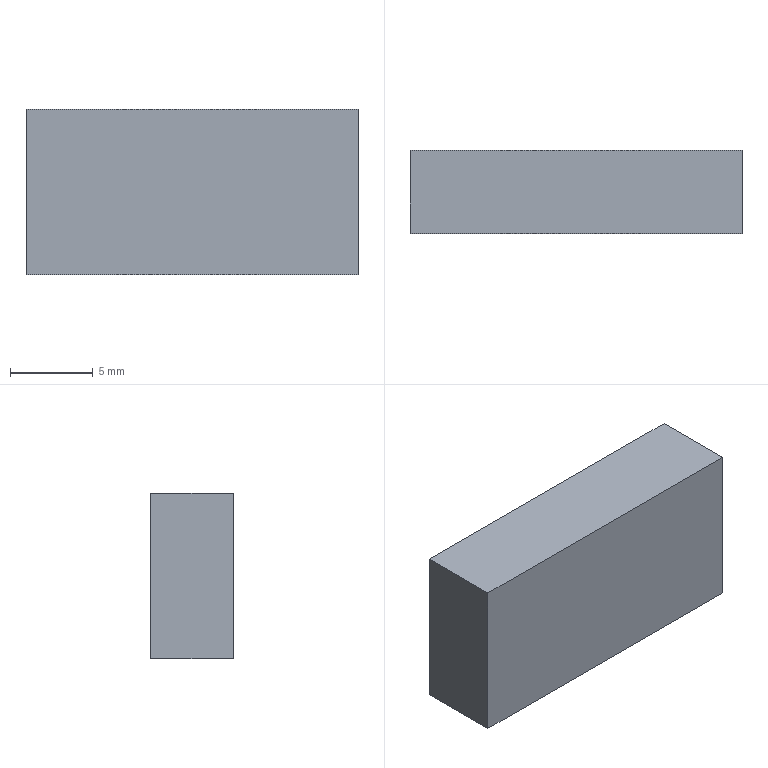Part | SolidWorks | features Extrusion 1 | 1 solid | 6 faces | box 20 x 5 x 10 mm | volume 1000 mm3 | plane 6
STEP:
#1=CARTESIAN_POINT('',(10.,0.,5.));
#2=VERTEX_POINT('',#1);
#3=CARTESIAN_POINT('',(10.,0.,-5.));
#4=VERTEX_POINT('',#3);
#5=CARTESIAN_POINT('',(10.,0.,5.));
#6=DIRECTION('',(0.,0.,-1.));
#7=VECTOR('',#6,1000.);
#8=LINE('',#5,#7);
#9=EDGE_CURVE('',#2,#4,#8,.T.);
#10=ORIENTED_EDGE('',*,*,#9,.T.);
#11=CARTESIAN_POINT('',(10.,5.,-5.));
#12=VERTEX_POINT('',#11);
#13=CARTESIAN_POINT('',(10.,5.,-5.));
#14=DIRECTION('',(0.,-1.,0.));
#15=VECTOR('',#14,1000.);
#16=LINE('',#13,#15);
#17=EDGE_CURVE('',#12,#4,#16,.T.);
#18=ORIENTED_EDGE('',*,*,#17,.F.);
#19=CARTESIAN_POINT('',(10.,5.,5.));
#20=VERTEX_POINT('',#19);
#21=CARTESIAN_POINT('',(10.,5.,5.));
#22=DIRECTION('',(0.,0.,-1.));
#23=VECTOR('',#22,1000.);
#24=LINE('',#21,#23);
#25=EDGE_CURVE('',#20,#12,#24,.T.);
#26=ORIENTED_EDGE('',*,*,#25,.F.);
#27=CARTESIAN_POINT('',(10.,5.,5.));
#28=DIRECTION('',(0.,-1.,0.));
#29=VECTOR('',#28,1000.);
#30=LINE('',#27,#29);
#31=EDGE_CURVE('',#20,#2,#30,.T.);
#32=ORIENTED_EDGE('',*,*,#31,.T.);
#33=EDGE_LOOP('',(#10,#18,#26,#32));
#34=FACE_OUTER_BOUND('',#33,.T.);
#35=CARTESIAN_POINT('',(10.,5.,5.));
#36=DIRECTION('',(-1.,0.,0.));
#37=DIRECTION('',(0.,0.,1.));
#38=AXIS2_PLACEMENT_3D('',#35,#36,#37);
#39=PLANE('',#38);
#40=ADVANCED_FACE('',(#34),#39,.F.);
#41=CARTESIAN_POINT('',(-10.,0.,-5.));
#42=VERTEX_POINT('',#41);
#43=CARTESIAN_POINT('',(-10.,0.,-5.));
#44=DIRECTION('',(-1.,0.,0.));
#45=VECTOR('',#44,1000.);
#46=LINE('',#43,#45);
#47=EDGE_CURVE('',#4,#42,#46,.T.);
#48=ORIENTED_EDGE('',*,*,#47,.T.);
#49=CARTESIAN_POINT('',(-10.,5.,-5.));
#50=VERTEX_POINT('',#49);
#51=CARTESIAN_POINT('',(-10.,5.,-5.));
#52=DIRECTION('',(0.,-1.,0.));
#53=VECTOR('',#52,1000.);
#54=LINE('',#51,#53);
#55=EDGE_CURVE('',#50,#42,#54,.T.);
#56=ORIENTED_EDGE('',*,*,#55,.F.);
#57=CARTESIAN_POINT('',(-10.,5.,-5.));
#58=DIRECTION('',(-1.,0.,0.));
#59=VECTOR('',#58,1000.);
#60=LINE('',#57,#59);
#61=EDGE_CURVE('',#12,#50,#60,.T.);
#62=ORIENTED_EDGE('',*,*,#61,.F.);
#63=ORIENTED_EDGE('',*,*,#17,.T.);
#64=EDGE_LOOP('',(#48,#56,#62,#63));
#65=FACE_OUTER_BOUND('',#64,.T.);
#66=CARTESIAN_POINT('',(-10.,5.,-5.));
#67=DIRECTION('',(0.,0.,1.));
#68=DIRECTION('',(1.,0.,0.));
#69=AXIS2_PLACEMENT_3D('',#66,#67,#68);
#70=PLANE('',#69);
#71=ADVANCED_FACE('',(#65),#70,.F.);
#72=CARTESIAN_POINT('',(-10.,0.,5.));
#73=VERTEX_POINT('',#72);
#74=CARTESIAN_POINT('',(-10.,0.,5.));
#75=DIRECTION('',(0.,0.,1.));
#76=VECTOR('',#75,1000.);
#77=LINE('',#74,#76);
#78=EDGE_CURVE('',#42,#73,#77,.T.);
#79=ORIENTED_EDGE('',*,*,#78,.T.);
#80=CARTESIAN_POINT('',(-10.,5.,5.));
#81=VERTEX_POINT('',#80);
#82=CARTESIAN_POINT('',(-10.,5.,5.));
#83=DIRECTION('',(0.,-1.,0.));
#84=VECTOR('',#83,1000.);
#85=LINE('',#82,#84);
#86=EDGE_CURVE('',#81,#73,#85,.T.);
#87=ORIENTED_EDGE('',*,*,#86,.F.);
#88=CARTESIAN_POINT('',(-10.,5.,5.));
#89=DIRECTION('',(0.,0.,1.));
#90=VECTOR('',#89,1000.);
#91=LINE('',#88,#90);
#92=EDGE_CURVE('',#50,#81,#91,.T.);
#93=ORIENTED_EDGE('',*,*,#92,.F.);
#94=ORIENTED_EDGE('',*,*,#55,.T.);
#95=EDGE_LOOP('',(#79,#87,#93,#94));
#96=FACE_OUTER_BOUND('',#95,.T.);
#97=CARTESIAN_POINT('',(-10.,5.,5.));
#98=DIRECTION('',(1.,0.,0.));
#99=DIRECTION('',(0.,0.,-1.));
#100=AXIS2_PLACEMENT_3D('',#97,#98,#99);
#101=PLANE('',#100);
#102=ADVANCED_FACE('',(#96),#101,.F.);
#103=CARTESIAN_POINT('',(-10.,0.,5.));
#104=DIRECTION('',(1.,0.,0.));
#105=VECTOR('',#104,1000.);
#106=LINE('',#103,#105);
#107=EDGE_CURVE('',#73,#2,#106,.T.);
#108=ORIENTED_EDGE('',*,*,#107,.T.);
#109=ORIENTED_EDGE('',*,*,#31,.F.);
#110=CARTESIAN_POINT('',(-10.,5.,5.));
#111=DIRECTION('',(1.,0.,0.));
#112=VECTOR('',#111,1000.);
#113=LINE('',#110,#112);
#114=EDGE_CURVE('',#81,#20,#113,.T.);
#115=ORIENTED_EDGE('',*,*,#114,.F.);
#116=ORIENTED_EDGE('',*,*,#86,.T.);
#117=EDGE_LOOP('',(#108,#109,#115,#116));
#118=FACE_OUTER_BOUND('',#117,.T.);
#119=CARTESIAN_POINT('',(-10.,5.,5.));
#120=DIRECTION('',(0.,0.,-1.));
#121=DIRECTION('',(-1.,0.,0.));
#122=AXIS2_PLACEMENT_3D('',#119,#120,#121);
#123=PLANE('',#122);
#124=ADVANCED_FACE('',(#118),#123,.F.);
#125=ORIENTED_EDGE('',*,*,#25,.T.);
#126=ORIENTED_EDGE('',*,*,#61,.T.);
#127=ORIENTED_EDGE('',*,*,#92,.T.);
#128=ORIENTED_EDGE('',*,*,#114,.T.);
#129=EDGE_LOOP('',(#125,#126,#127,#128));
#130=FACE_OUTER_BOUND('',#129,.T.);
#131=CARTESIAN_POINT('',(0.,5.,0.));
#132=DIRECTION('',(0.,-1.,0.));
#133=DIRECTION('',(0.,0.,-1.));
#134=AXIS2_PLACEMENT_3D('',#131,#132,#133);
#135=PLANE('',#134);
#136=ADVANCED_FACE('',(#130),#135,.F.);
#137=ORIENTED_EDGE('',*,*,#9,.F.);
#138=ORIENTED_EDGE('',*,*,#107,.F.);
#139=ORIENTED_EDGE('',*,*,#78,.F.);
#140=ORIENTED_EDGE('',*,*,#47,.F.);
#141=EDGE_LOOP('',(#137,#138,#139,#140));
#142=FACE_OUTER_BOUND('',#141,.T.);
#143=CARTESIAN_POINT('',(0.,0.,0.));
#144=DIRECTION('',(0.,-1.,0.));
#145=DIRECTION('',(0.,0.,-1.));
#146=AXIS2_PLACEMENT_3D('',#143,#144,#145);
#147=PLANE('',#146);
#148=ADVANCED_FACE('',(#142),#147,.T.);
#149=CLOSED_SHELL('',(#40,#71,#102,#124,#136,#148));
#150=MANIFOLD_SOLID_BREP('',#149);
#151=CARTESIAN_POINT('',(0.,0.,0.));
#152=DIRECTION('',(0.,0.,1.));
#153=DIRECTION('',(1.,0.,0.));
#154=AXIS2_PLACEMENT_3D('',#151,#152,#153);
#155=(LENGTH_UNIT()NAMED_UNIT(*)SI_UNIT(.MILLI.,.METRE.));
#156=UNCERTAINTY_MEASURE_WITH_UNIT(LENGTH_MEASURE(0.00001),#155,'','');
#157=(NAMED_UNIT(*)PLANE_ANGLE_UNIT()SI_UNIT($,.RADIAN.));
#158=(NAMED_UNIT(*)SI_UNIT($,.STERADIAN.)SOLID_ANGLE_UNIT());
#159=(GEOMETRIC_REPRESENTATION_CONTEXT(3)GLOBAL_UNCERTAINTY_ASSIGNED_CONTEXT((#156))GLOBAL_UNIT_ASSIGNED_CONTEXT((#155,#157,#158))REPRESENTATION_CONTEXT('',''));
#160=ADVANCED_BREP_SHAPE_REPRESENTATION('',(#150,#154),#159);